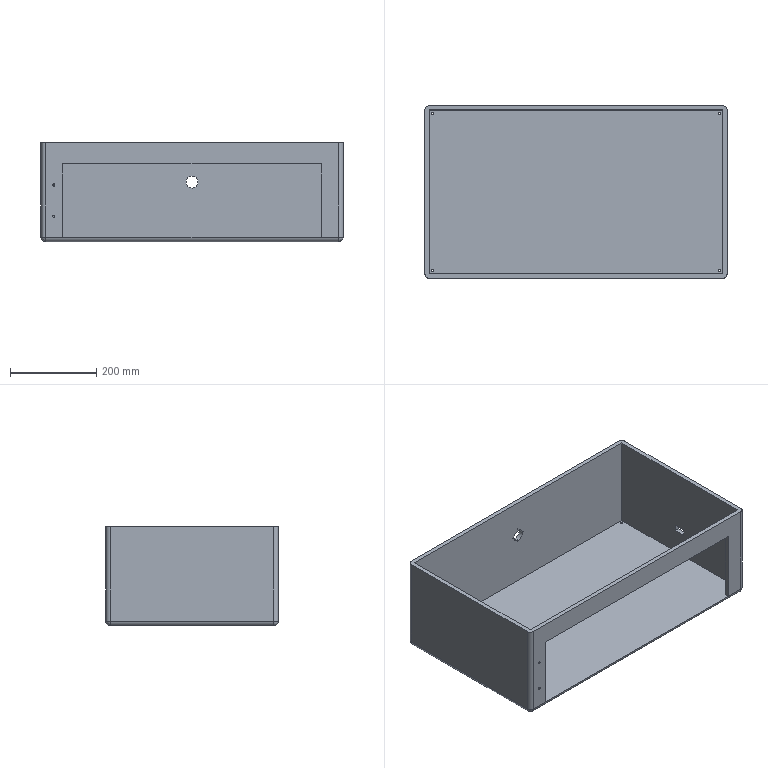Part | SolidWorks | features Cut 4, HoleWzd 3, Extrusion 1, Fillet 1, Shell 1 | 1 solid | 68 faces | box 700 x 400 x 230 mm | volume 6454208 mm3 | cylinder 34 | plane 18 | cone 12 | sphere 4 | commonest cylinder face diameters 5 x12 2.5 x8 20 x8 2.05 x4 28 x2